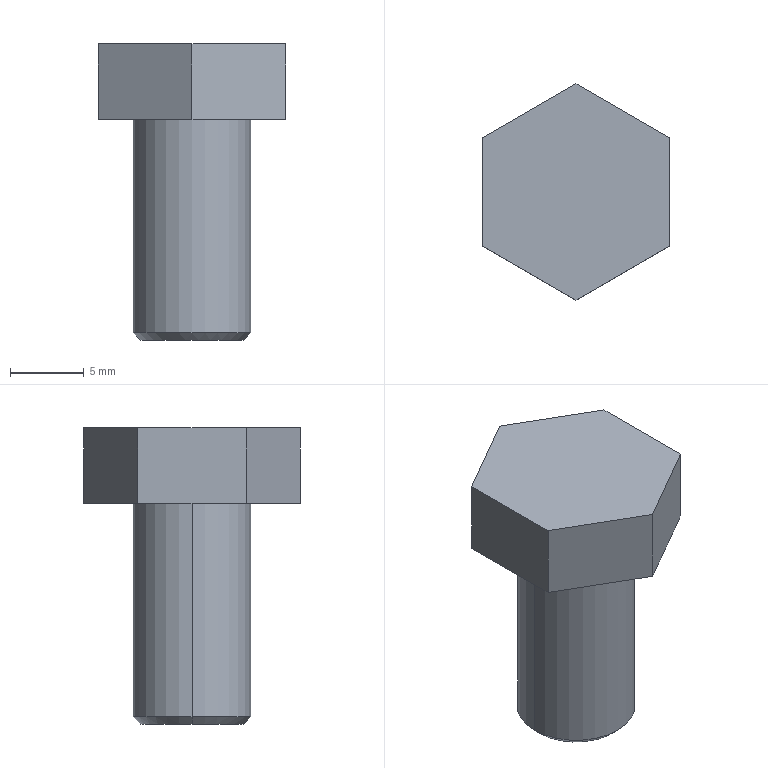Part | STEP file | Bulong M8_1.5F | 1 solid | 13 faces | box 12.73 x 14.699 x 20.15 mm | volume 1474 mm3 | plane 9 | cone 2 | cylinder 2 | commonest cylinder face diameters 8 x2
STEP:
#1=CARTESIAN_POINT('',(0.,0.,0.));
#2=DIRECTION('',(0.,0.,1.));
#3=DIRECTION('',(1.,0.,0.));
#4=AXIS2_PLACEMENT_3D('',#1,#2,#3);
#5=CARTESIAN_POINT('',(-3.5,0.,-15.));
#6=VERTEX_POINT('',#5);
#7=CARTESIAN_POINT('',(3.5,0.,-15.));
#8=VERTEX_POINT('',#7);
#9=CARTESIAN_POINT('',(0.,0.,-15.));
#10=DIRECTION('',(0.,0.,-1.));
#11=DIRECTION('',(-1.,0.,0.));
#12=AXIS2_PLACEMENT_3D('',#9,#10,#11);
#13=CIRCLE('',#12,3.5);
#14=CARTESIAN_POINT('',(0.,0.,-15.));
#15=DIRECTION('',(0.,0.,1.));
#16=DIRECTION('',(1.,0.,0.));
#17=AXIS2_PLACEMENT_3D('',#14,#15,#16);
#18=CONICAL_SURFACE('',#17,3.5,0.7854);
#19=CARTESIAN_POINT('',(3.142,0.));
#20=DIRECTION('',(-1.,0.));
#21=VECTOR('',#20,1.);
#22=LINE('',#19,#21);
#23=(GEOMETRIC_REPRESENTATION_CONTEXT(2)PARAMETRIC_REPRESENTATION_CONTEXT()REPRESENTATION_CONTEXT('',''));
#24=DEFINITIONAL_REPRESENTATION('',(#22),#23);
#25=PCURVE('',#18,#24);
#26=CARTESIAN_POINT('',(0.,0.,-15.));
#27=DIRECTION('',(0.,0.,-1.));
#28=DIRECTION('',(-1.,0.,0.));
#29=AXIS2_PLACEMENT_3D('',#26,#27,#28);
#30=PLANE('',#29);
#31=CARTESIAN_POINT('',(0.,0.));
#32=DIRECTION('',(1.,0.));
#33=AXIS2_PLACEMENT_2D('',#31,#32);
#34=CIRCLE('',#33,3.5);
#35=(GEOMETRIC_REPRESENTATION_CONTEXT(2)PARAMETRIC_REPRESENTATION_CONTEXT()REPRESENTATION_CONTEXT('',''));
#36=DEFINITIONAL_REPRESENTATION('',(#34),#35);
#37=PCURVE('',#30,#36);
#38=SURFACE_CURVE('',#13,(#25,#37),.PCURVE_S1.);
#39=EDGE_CURVE('',#6,#8,#38,.T.);
#40=ORIENTED_EDGE('',*,*,#39,.F.);
#41=CARTESIAN_POINT('',(-4.,0.,-14.5));
#42=VERTEX_POINT('',#41);
#43=CARTESIAN_POINT('',(-3.5,0.,-15.));
#44=DIRECTION('',(-0.7071,0.,0.7071));
#45=VECTOR('',#44,1.);
#46=LINE('',#43,#45);
#47=CARTESIAN_POINT('',(3.142,0.));
#48=DIRECTION('',(0.,1.));
#49=VECTOR('',#48,1.);
#50=LINE('',#47,#49);
#51=(GEOMETRIC_REPRESENTATION_CONTEXT(2)PARAMETRIC_REPRESENTATION_CONTEXT()REPRESENTATION_CONTEXT('',''));
#52=DEFINITIONAL_REPRESENTATION('',(#50),#51);
#53=PCURVE('',#18,#52);
#54=CARTESIAN_POINT('',(0.,0.,-15.));
#55=DIRECTION('',(0.,0.,1.));
#56=DIRECTION('',(1.,0.,0.));
#57=AXIS2_PLACEMENT_3D('',#54,#55,#56);
#58=CONICAL_SURFACE('',#57,3.5,0.7854);
#59=CARTESIAN_POINT('',(3.142,0.));
#60=DIRECTION('',(0.,1.));
#61=VECTOR('',#60,1.);
#62=LINE('',#59,#61);
#63=(GEOMETRIC_REPRESENTATION_CONTEXT(2)PARAMETRIC_REPRESENTATION_CONTEXT()REPRESENTATION_CONTEXT('',''));
#64=DEFINITIONAL_REPRESENTATION('',(#62),#63);
#65=PCURVE('',#58,#64);
#66=SURFACE_CURVE('',#46,(#53,#65),.PCURVE_S1.);
#67=EDGE_CURVE('',#6,#42,#66,.T.);
#68=ORIENTED_EDGE('',*,*,#67,.T.);
#69=CARTESIAN_POINT('',(4.,0.,-14.5));
#70=VERTEX_POINT('',#69);
#71=CARTESIAN_POINT('',(0.,0.,-14.5));
#72=DIRECTION('',(0.,0.,1.));
#73=DIRECTION('',(-1.,0.,0.));
#74=AXIS2_PLACEMENT_3D('',#71,#72,#73);
#75=CIRCLE('',#74,4.);
#76=CARTESIAN_POINT('',(-3.142,0.5));
#77=DIRECTION('',(1.,0.));
#78=VECTOR('',#77,1.);
#79=LINE('',#76,#78);
#80=(GEOMETRIC_REPRESENTATION_CONTEXT(2)PARAMETRIC_REPRESENTATION_CONTEXT()REPRESENTATION_CONTEXT('',''));
#81=DEFINITIONAL_REPRESENTATION('',(#79),#80);
#82=PCURVE('',#18,#81);
#83=CARTESIAN_POINT('',(0.,0.,-15.));
#84=DIRECTION('',(0.,0.,1.));
#85=DIRECTION('',(1.,0.,0.));
#86=AXIS2_PLACEMENT_3D('',#83,#84,#85);
#87=CYLINDRICAL_SURFACE('',#86,4.);
#88=CARTESIAN_POINT('',(-3.142,0.5));
#89=DIRECTION('',(1.,0.));
#90=VECTOR('',#89,1.);
#91=LINE('',#88,#90);
#92=(GEOMETRIC_REPRESENTATION_CONTEXT(2)PARAMETRIC_REPRESENTATION_CONTEXT()REPRESENTATION_CONTEXT('',''));
#93=DEFINITIONAL_REPRESENTATION('',(#91),#92);
#94=PCURVE('',#87,#93);
#95=SURFACE_CURVE('',#75,(#82,#94),.PCURVE_S1.);
#96=EDGE_CURVE('',#70,#42,#95,.T.);
#97=ORIENTED_EDGE('',*,*,#96,.F.);
#98=CARTESIAN_POINT('',(3.5,0.,-15.));
#99=DIRECTION('',(0.7071,0.,0.7071));
#100=VECTOR('',#99,1.);
#101=LINE('',#98,#100);
#102=CARTESIAN_POINT('',(0.,0.));
#103=DIRECTION('',(0.,1.));
#104=VECTOR('',#103,1.);
#105=LINE('',#102,#104);
#106=(GEOMETRIC_REPRESENTATION_CONTEXT(2)PARAMETRIC_REPRESENTATION_CONTEXT()REPRESENTATION_CONTEXT('',''));
#107=DEFINITIONAL_REPRESENTATION('',(#105),#106);
#108=PCURVE('',#18,#107);
#109=CARTESIAN_POINT('',(6.283,0.));
#110=DIRECTION('',(0.,1.));
#111=VECTOR('',#110,1.);
#112=LINE('',#109,#111);
#113=(GEOMETRIC_REPRESENTATION_CONTEXT(2)PARAMETRIC_REPRESENTATION_CONTEXT()REPRESENTATION_CONTEXT('',''));
#114=DEFINITIONAL_REPRESENTATION('',(#112),#113);
#115=PCURVE('',#58,#114);
#116=SURFACE_CURVE('',#101,(#108,#115),.PCURVE_S1.);
#117=EDGE_CURVE('',#8,#70,#116,.T.);
#118=ORIENTED_EDGE('',*,*,#117,.F.);
#119=EDGE_LOOP('',(#40,#68,#97,#118));
#120=FACE_BOUND('',#119,.T.);
#121=ADVANCED_FACE('',(#120),#18,.T.);
#122=ORIENTED_EDGE('',*,*,#96,.T.);
#123=CARTESIAN_POINT('',(-4.,0.,0.));
#124=VERTEX_POINT('',#123);
#125=CARTESIAN_POINT('',(-4.,0.,-15.));
#126=DIRECTION('',(0.,0.,1.));
#127=VECTOR('',#126,1.);
#128=LINE('',#125,#127);
#129=CARTESIAN_POINT('',(3.142,0.));
#130=DIRECTION('',(0.,1.));
#131=VECTOR('',#130,1.);
#132=LINE('',#129,#131);
#133=(GEOMETRIC_REPRESENTATION_CONTEXT(2)PARAMETRIC_REPRESENTATION_CONTEXT()REPRESENTATION_CONTEXT('',''));
#134=DEFINITIONAL_REPRESENTATION('',(#132),#133);
#135=PCURVE('',#87,#134);
#136=CARTESIAN_POINT('',(0.,0.,-15.));
#137=DIRECTION('',(0.,0.,1.));
#138=DIRECTION('',(1.,0.,0.));
#139=AXIS2_PLACEMENT_3D('',#136,#137,#138);
#140=CYLINDRICAL_SURFACE('',#139,4.);
#141=CARTESIAN_POINT('',(3.142,0.));
#142=DIRECTION('',(0.,1.));
#143=VECTOR('',#142,1.);
#144=LINE('',#141,#143);
#145=(GEOMETRIC_REPRESENTATION_CONTEXT(2)PARAMETRIC_REPRESENTATION_CONTEXT()REPRESENTATION_CONTEXT('',''));
#146=DEFINITIONAL_REPRESENTATION('',(#144),#145);
#147=PCURVE('',#140,#146);
#148=SURFACE_CURVE('',#128,(#135,#147),.PCURVE_S1.);
#149=EDGE_CURVE('',#42,#124,#148,.T.);
#150=ORIENTED_EDGE('',*,*,#149,.T.);
#151=CARTESIAN_POINT('',(4.,0.,0.));
#152=VERTEX_POINT('',#151);
#153=CARTESIAN_POINT('',(0.,0.,0.));
#154=DIRECTION('',(0.,0.,-1.));
#155=DIRECTION('',(1.,0.,0.));
#156=AXIS2_PLACEMENT_3D('',#153,#154,#155);
#157=CIRCLE('',#156,4.);
#158=CARTESIAN_POINT('',(6.283,15.));
#159=DIRECTION('',(-1.,0.));
#160=VECTOR('',#159,1.);
#161=LINE('',#158,#160);
#162=(GEOMETRIC_REPRESENTATION_CONTEXT(2)PARAMETRIC_REPRESENTATION_CONTEXT()REPRESENTATION_CONTEXT('',''));
#163=DEFINITIONAL_REPRESENTATION('',(#161),#162);
#164=PCURVE('',#87,#163);
#165=CARTESIAN_POINT('',(0.,0.,0.));
#166=DIRECTION('',(0.,0.,1.));
#167=DIRECTION('',(1.,0.,0.));
#168=AXIS2_PLACEMENT_3D('',#165,#166,#167);
#169=PLANE('',#168);
#170=CARTESIAN_POINT('',(4.,0.));
#171=CARTESIAN_POINT('',(4.,-6.928));
#172=CARTESIAN_POINT('',(-2.,-3.464));
#173=CARTESIAN_POINT('',(-8.,0.));
#174=CARTESIAN_POINT('',(-2.,3.464));
#175=CARTESIAN_POINT('',(4.,6.928));
#176=CARTESIAN_POINT('',(4.,0.));
#177=(BOUNDED_CURVE()B_SPLINE_CURVE(2,(#170,#171,#172,#173,#174,#175,#176),.UNSPECIFIED.,.T.,.F.)B_SPLINE_CURVE_WITH_KNOTS((1,2,2,2,2,1),(-2.094,0.,2.094,4.189,6.283,8.378),.UNSPECIFIED.)CURVE()GEOMETRIC_REPRESENTATION_ITEM()RATIONAL_B_SPLINE_CURVE((1.,0.5,1.,0.5,1.,0.5,1.))REPRESENTATION_ITEM(''));
#178=(GEOMETRIC_REPRESENTATION_CONTEXT(2)PARAMETRIC_REPRESENTATION_CONTEXT()REPRESENTATION_CONTEXT('',''));
#179=DEFINITIONAL_REPRESENTATION('',(#177),#178);
#180=PCURVE('',#169,#179);
#181=SURFACE_CURVE('',#157,(#164,#180),.PCURVE_S1.);
#182=EDGE_CURVE('',#124,#152,#181,.T.);
#183=ORIENTED_EDGE('',*,*,#182,.T.);
#184=CARTESIAN_POINT('',(4.,0.,-15.));
#185=DIRECTION('',(0.,0.,1.));
#186=VECTOR('',#185,1.);
#187=LINE('',#184,#186);
#188=CARTESIAN_POINT('',(0.,0.));
#189=DIRECTION('',(0.,1.));
#190=VECTOR('',#189,1.);
#191=LINE('',#188,#190);
#192=(GEOMETRIC_REPRESENTATION_CONTEXT(2)PARAMETRIC_REPRESENTATION_CONTEXT()REPRESENTATION_CONTEXT('',''));
#193=DEFINITIONAL_REPRESENTATION('',(#191),#192);
#194=PCURVE('',#87,#193);
#195=CARTESIAN_POINT('',(6.283,0.));
#196=DIRECTION('',(0.,1.));
#197=VECTOR('',#196,1.);
#198=LINE('',#195,#197);
#199=(GEOMETRIC_REPRESENTATION_CONTEXT(2)PARAMETRIC_REPRESENTATION_CONTEXT()REPRESENTATION_CONTEXT('',''));
#200=DEFINITIONAL_REPRESENTATION('',(#198),#199);
#201=PCURVE('',#140,#200);
#202=SURFACE_CURVE('',#187,(#194,#201),.PCURVE_S1.);
#203=EDGE_CURVE('',#70,#152,#202,.T.);
#204=ORIENTED_EDGE('',*,*,#203,.F.);
#205=EDGE_LOOP('',(#122,#150,#183,#204));
#206=FACE_BOUND('',#205,.T.);
#207=ADVANCED_FACE('',(#206),#87,.T.);
#208=CARTESIAN_POINT('',(6.365,3.675,0.));
#209=VERTEX_POINT('',#208);
#210=CARTESIAN_POINT('',(0.,7.35,0.));
#211=VERTEX_POINT('',#210);
#212=CARTESIAN_POINT('',(6.365,3.675,0.));
#213=DIRECTION('',(-0.866,0.5,0.));
#214=VECTOR('',#213,1.);
#215=LINE('',#212,#214);
#216=CARTESIAN_POINT('',(6.365,3.675));
#217=DIRECTION('',(-0.866,0.5));
#218=VECTOR('',#217,1.);
#219=LINE('',#216,#218);
#220=(GEOMETRIC_REPRESENTATION_CONTEXT(2)PARAMETRIC_REPRESENTATION_CONTEXT()REPRESENTATION_CONTEXT('',''));
#221=DEFINITIONAL_REPRESENTATION('',(#219),#220);
#222=PCURVE('',#169,#221);
#223=CARTESIAN_POINT('',(6.365,3.675,5.15));
#224=DIRECTION('',(-0.5,-0.866,0.));
#225=DIRECTION('',(0.866,-0.5,0.));
#226=AXIS2_PLACEMENT_3D('',#223,#224,#225);
#227=PLANE('',#226);
#228=CARTESIAN_POINT('',(0.,-5.15));
#229=DIRECTION('',(-1.,0.));
#230=VECTOR('',#229,1.);
#231=LINE('',#228,#230);
#232=(GEOMETRIC_REPRESENTATION_CONTEXT(2)PARAMETRIC_REPRESENTATION_CONTEXT()REPRESENTATION_CONTEXT('',''));
#233=DEFINITIONAL_REPRESENTATION('',(#231),#232);
#234=PCURVE('',#227,#233);
#235=SURFACE_CURVE('',#215,(#222,#234),.PCURVE_S1.);
#236=EDGE_CURVE('',#209,#211,#235,.T.);
#237=ORIENTED_EDGE('',*,*,#236,.F.);
#238=CARTESIAN_POINT('',(6.365,-3.675,0.));
#239=VERTEX_POINT('',#238);
#240=CARTESIAN_POINT('',(6.365,-3.675,0.));
#241=DIRECTION('',(0.,1.,0.));
#242=VECTOR('',#241,1.);
#243=LINE('',#240,#242);
#244=CARTESIAN_POINT('',(6.365,-3.675));
#245=DIRECTION('',(0.,1.));
#246=VECTOR('',#245,1.);
#247=LINE('',#244,#246);
#248=(GEOMETRIC_REPRESENTATION_CONTEXT(2)PARAMETRIC_REPRESENTATION_CONTEXT()REPRESENTATION_CONTEXT('',''));
#249=DEFINITIONAL_REPRESENTATION('',(#247),#248);
#250=PCURVE('',#169,#249);
#251=CARTESIAN_POINT('',(6.365,-3.675,5.15));
#252=DIRECTION('',(-1.,0.,0.));
#253=DIRECTION('',(0.,-1.,0.));
#254=AXIS2_PLACEMENT_3D('',#251,#252,#253);
#255=PLANE('',#254);
#256=CARTESIAN_POINT('',(0.,-5.15));
#257=DIRECTION('',(-1.,0.));
#258=VECTOR('',#257,1.);
#259=LINE('',#256,#258);
#260=(GEOMETRIC_REPRESENTATION_CONTEXT(2)PARAMETRIC_REPRESENTATION_CONTEXT()REPRESENTATION_CONTEXT('',''));
#261=DEFINITIONAL_REPRESENTATION('',(#259),#260);
#262=PCURVE('',#255,#261);
#263=SURFACE_CURVE('',#243,(#250,#262),.PCURVE_S1.);
#264=EDGE_CURVE('',#239,#209,#263,.T.);
#265=ORIENTED_EDGE('',*,*,#264,.F.);
#266=CARTESIAN_POINT('',(0.,-7.35,0.));
#267=VERTEX_POINT('',#266);
#268=CARTESIAN_POINT('',(0.,-7.35,0.));
#269=DIRECTION('',(0.866,0.5,0.));
#270=VECTOR('',#269,1.);
#271=LINE('',#268,#270);
#272=CARTESIAN_POINT('',(0.,-7.35));
#273=DIRECTION('',(0.866,0.5));
#274=VECTOR('',#273,1.);
#275=LINE('',#272,#274);
#276=(GEOMETRIC_REPRESENTATION_CONTEXT(2)PARAMETRIC_REPRESENTATION_CONTEXT()REPRESENTATION_CONTEXT('',''));
#277=DEFINITIONAL_REPRESENTATION('',(#275),#276);
#278=PCURVE('',#169,#277);
#279=CARTESIAN_POINT('',(0.,-7.35,5.15));
#280=DIRECTION('',(-0.5,0.866,0.));
#281=DIRECTION('',(-0.866,-0.5,0.));
#282=AXIS2_PLACEMENT_3D('',#279,#280,#281);
#283=PLANE('',#282);
#284=CARTESIAN_POINT('',(0.,-5.15));
#285=DIRECTION('',(-1.,0.));
#286=VECTOR('',#285,1.);
#287=LINE('',#284,#286);
#288=(GEOMETRIC_REPRESENTATION_CONTEXT(2)PARAMETRIC_REPRESENTATION_CONTEXT()REPRESENTATION_CONTEXT('',''));
#289=DEFINITIONAL_REPRESENTATION('',(#287),#288);
#290=PCURVE('',#283,#289);
#291=SURFACE_CURVE('',#271,(#278,#290),.PCURVE_S1.);
#292=EDGE_CURVE('',#267,#239,#291,.T.);
#293=ORIENTED_EDGE('',*,*,#292,.F.);
#294=CARTESIAN_POINT('',(-6.365,-3.675,0.));
#295=VERTEX_POINT('',#294);
#296=CARTESIAN_POINT('',(-6.365,-3.675,0.));
#297=DIRECTION('',(0.866,-0.5,0.));
#298=VECTOR('',#297,1.);
#299=LINE('',#296,#298);
#300=CARTESIAN_POINT('',(-6.365,-3.675));
#301=DIRECTION('',(0.866,-0.5));
#302=VECTOR('',#301,1.);
#303=LINE('',#300,#302);
#304=(GEOMETRIC_REPRESENTATION_CONTEXT(2)PARAMETRIC_REPRESENTATION_CONTEXT()REPRESENTATION_CONTEXT('',''));
#305=DEFINITIONAL_REPRESENTATION('',(#303),#304);
#306=PCURVE('',#169,#305);
#307=CARTESIAN_POINT('',(-6.365,-3.675,5.15));
#308=DIRECTION('',(0.5,0.866,0.));
#309=DIRECTION('',(-0.866,0.5,0.));
#310=AXIS2_PLACEMENT_3D('',#307,#308,#309);
#311=PLANE('',#310);
#312=CARTESIAN_POINT('',(0.,-5.15));
#313=DIRECTION('',(-1.,0.));
#314=VECTOR('',#313,1.);
#315=LINE('',#312,#314);
#316=(GEOMETRIC_REPRESENTATION_CONTEXT(2)PARAMETRIC_REPRESENTATION_CONTEXT()REPRESENTATION_CONTEXT('',''));
#317=DEFINITIONAL_REPRESENTATION('',(#315),#316);
#318=PCURVE('',#311,#317);
#319=SURFACE_CURVE('',#299,(#306,#318),.PCURVE_S1.);
#320=EDGE_CURVE('',#295,#267,#319,.T.);
#321=ORIENTED_EDGE('',*,*,#320,.F.);
#322=CARTESIAN_POINT('',(-6.365,3.675,0.));
#323=VERTEX_POINT('',#322);
#324=CARTESIAN_POINT('',(-6.365,3.675,0.));
#325=DIRECTION('',(0.,-1.,0.));
#326=VECTOR('',#325,1.);
#327=LINE('',#324,#326);
#328=CARTESIAN_POINT('',(-6.365,3.675));
#329=DIRECTION('',(0.,-1.));
#330=VECTOR('',#329,1.);
#331=LINE('',#328,#330);
#332=(GEOMETRIC_REPRESENTATION_CONTEXT(2)PARAMETRIC_REPRESENTATION_CONTEXT()REPRESENTATION_CONTEXT('',''));
#333=DEFINITIONAL_REPRESENTATION('',(#331),#332);
#334=PCURVE('',#169,#333);
#335=CARTESIAN_POINT('',(-6.365,3.675,5.15));
#336=DIRECTION('',(1.,0.,0.));
#337=DIRECTION('',(0.,0.,-1.));
#338=AXIS2_PLACEMENT_3D('',#335,#336,#337);
#339=PLANE('',#338);
#340=CARTESIAN_POINT('',(5.15,0.));
#341=DIRECTION('',(0.,-1.));
#342=VECTOR('',#341,1.);
#343=LINE('',#340,#342);
#344=(GEOMETRIC_REPRESENTATION_CONTEXT(2)PARAMETRIC_REPRESENTATION_CONTEXT()REPRESENTATION_CONTEXT('',''));
#345=DEFINITIONAL_REPRESENTATION('',(#343),#344);
#346=PCURVE('',#339,#345);
#347=SURFACE_CURVE('',#327,(#334,#346),.PCURVE_S1.);
#348=EDGE_CURVE('',#323,#295,#347,.T.);
#349=ORIENTED_EDGE('',*,*,#348,.F.);
#350=CARTESIAN_POINT('',(0.,7.35,0.));
#351=DIRECTION('',(-0.866,-0.5,0.));
#352=VECTOR('',#351,1.);
#353=LINE('',#350,#352);
#354=CARTESIAN_POINT('',(0.,7.35));
#355=DIRECTION('',(-0.866,-0.5));
#356=VECTOR('',#355,1.);
#357=LINE('',#354,#356);
#358=(GEOMETRIC_REPRESENTATION_CONTEXT(2)PARAMETRIC_REPRESENTATION_CONTEXT()REPRESENTATION_CONTEXT('',''));
#359=DEFINITIONAL_REPRESENTATION('',(#357),#358);
#360=PCURVE('',#169,#359);
#361=CARTESIAN_POINT('',(0.,7.35,5.15));
#362=DIRECTION('',(0.5,-0.866,0.));
#363=DIRECTION('',(0.866,0.5,0.));
#364=AXIS2_PLACEMENT_3D('',#361,#362,#363);
#365=PLANE('',#364);
#366=CARTESIAN_POINT('',(0.,-5.15));
#367=DIRECTION('',(-1.,0.));
#368=VECTOR('',#367,1.);
#369=LINE('',#366,#368);
#370=(GEOMETRIC_REPRESENTATION_CONTEXT(2)PARAMETRIC_REPRESENTATION_CONTEXT()REPRESENTATION_CONTEXT('',''));
#371=DEFINITIONAL_REPRESENTATION('',(#369),#370);
#372=PCURVE('',#365,#371);
#373=SURFACE_CURVE('',#353,(#360,#372),.PCURVE_S1.);
#374=EDGE_CURVE('',#211,#323,#373,.T.);
#375=ORIENTED_EDGE('',*,*,#374,.F.);
#376=EDGE_LOOP('',(#237,#265,#293,#321,#349,#375));
#377=FACE_BOUND('',#376,.T.);
#378=CARTESIAN_POINT('',(0.,0.,0.));
#379=DIRECTION('',(0.,0.,-1.));
#380=DIRECTION('',(1.,0.,0.));
#381=AXIS2_PLACEMENT_3D('',#378,#379,#380);
#382=CIRCLE('',#381,4.);
#383=CARTESIAN_POINT('',(4.,0.));
#384=CARTESIAN_POINT('',(4.,-6.928));
#385=CARTESIAN_POINT('',(-2.,-3.464));
#386=CARTESIAN_POINT('',(-8.,0.));
#387=CARTESIAN_POINT('',(-2.,3.464));
#388=CARTESIAN_POINT('',(4.,6.928));
#389=CARTESIAN_POINT('',(4.,0.));
#390=(BOUNDED_CURVE()B_SPLINE_CURVE(2,(#383,#384,#385,#386,#387,#388,#389),.UNSPECIFIED.,.T.,.F.)B_SPLINE_CURVE_WITH_KNOTS((1,2,2,2,2,1),(-2.094,0.,2.094,4.189,6.283,8.378),.UNSPECIFIED.)CURVE()GEOMETRIC_REPRESENTATION_ITEM()RATIONAL_B_SPLINE_CURVE((1.,0.5,1.,0.5,1.,0.5,1.))REPRESENTATION_ITEM(''));
#391=(GEOMETRIC_REPRESENTATION_CONTEXT(2)PARAMETRIC_REPRESENTATION_CONTEXT()REPRESENTATION_CONTEXT('',''));
#392=DEFINITIONAL_REPRESENTATION('',(#390),#391);
#393=PCURVE('',#169,#392);
#394=CARTESIAN_POINT('',(6.283,15.));
#395=DIRECTION('',(-1.,0.));
#396=VECTOR('',#395,1.);
#397=LINE('',#394,#396);
#398=(GEOMETRIC_REPRESENTATION_CONTEXT(2)PARAMETRIC_REPRESENTATION_CONTEXT()REPRESENTATION_CONTEXT('',''));
#399=DEFINITIONAL_REPRESENTATION('',(#397),#398);
#400=PCURVE('',#140,#399);
#401=SURFACE_CURVE('',#382,(#393,#400),.PCURVE_S1.);
#402=EDGE_CURVE('',#152,#124,#401,.T.);
#403=ORIENTED_EDGE('',*,*,#402,.F.);
#404=ORIENTED_EDGE('',*,*,#182,.F.);
#405=EDGE_LOOP('',(#403,#404));
#406=FACE_BOUND('',#405,.T.);
#407=ADVANCED_FACE('',(#377,#406),#169,.F.);
#408=ORIENTED_EDGE('',*,*,#236,.T.);
#409=CARTESIAN_POINT('',(0.,7.35,5.15));
#410=VERTEX_POINT('',#409);
#411=CARTESIAN_POINT('',(0.,7.35,5.15));
#412=DIRECTION('',(0.,0.,-1.));
#413=VECTOR('',#412,1.);
#414=LINE('',#411,#413);
#415=CARTESIAN_POINT('',(-7.35,0.));
#416=DIRECTION('',(0.,-1.));
#417=VECTOR('',#416,1.);
#418=LINE('',#415,#417);
#419=(GEOMETRIC_REPRESENTATION_CONTEXT(2)PARAMETRIC_REPRESENTATION_CONTEXT()REPRESENTATION_CONTEXT('',''));
#420=DEFINITIONAL_REPRESENTATION('',(#418),#419);
#421=PCURVE('',#227,#420);
#422=CARTESIAN_POINT('',(0.,0.));
#423=DIRECTION('',(0.,-1.));
#424=VECTOR('',#423,1.);
#425=LINE('',#422,#424);
#426=(GEOMETRIC_REPRESENTATION_CONTEXT(2)PARAMETRIC_REPRESENTATION_CONTEXT()REPRESENTATION_CONTEXT('',''));
#427=DEFINITIONAL_REPRESENTATION('',(#425),#426);
#428=PCURVE('',#365,#427);
#429=SURFACE_CURVE('',#414,(#421,#428),.PCURVE_S1.);
#430=EDGE_CURVE('',#410,#211,#429,.T.);
#431=ORIENTED_EDGE('',*,*,#430,.F.);
#432=CARTESIAN_POINT('',(6.365,3.675,5.15));
#433=VERTEX_POINT('',#432);
#434=CARTESIAN_POINT('',(6.365,3.675,5.15));
#435=DIRECTION('',(-0.866,0.5,0.));
#436=VECTOR('',#435,1.);
#437=LINE('',#434,#436);
#438=CARTESIAN_POINT('',(0.,0.));
#439=DIRECTION('',(-1.,0.));
#440=VECTOR('',#439,1.);
#441=LINE('',#438,#440);
#442=(GEOMETRIC_REPRESENTATION_CONTEXT(2)PARAMETRIC_REPRESENTATION_CONTEXT()REPRESENTATION_CONTEXT('',''));
#443=DEFINITIONAL_REPRESENTATION('',(#441),#442);
#444=PCURVE('',#227,#443);
#445=CARTESIAN_POINT('',(0.,0.,5.15));
#446=DIRECTION('',(0.,0.,1.));
#447=DIRECTION('',(1.,0.,0.));
#448=AXIS2_PLACEMENT_3D('',#445,#446,#447);
#449=PLANE('',#448);
#450=CARTESIAN_POINT('',(6.365,3.675));
#451=DIRECTION('',(-0.866,0.5));
#452=VECTOR('',#451,1.);
#453=LINE('',#450,#452);
#454=(GEOMETRIC_REPRESENTATION_CONTEXT(2)PARAMETRIC_REPRESENTATION_CONTEXT()REPRESENTATION_CONTEXT('',''));
#455=DEFINITIONAL_REPRESENTATION('',(#453),#454);
#456=PCURVE('',#449,#455);
#457=SURFACE_CURVE('',#437,(#444,#456),.PCURVE_S1.);
#458=EDGE_CURVE('',#433,#410,#457,.T.);
#459=ORIENTED_EDGE('',*,*,#458,.F.);
#460=CARTESIAN_POINT('',(6.365,3.675,5.15));
#461=DIRECTION('',(0.,0.,-1.));
#462=VECTOR('',#461,1.);
#463=LINE('',#460,#462);
#464=CARTESIAN_POINT('',(0.,0.));
#465=DIRECTION('',(0.,-1.));
#466=VECTOR('',#465,1.);
#467=LINE('',#464,#466);
#468=(GEOMETRIC_REPRESENTATION_CONTEXT(2)PARAMETRIC_REPRESENTATION_CONTEXT()REPRESENTATION_CONTEXT('',''));
#469=DEFINITIONAL_REPRESENTATION('',(#467),#468);
#470=PCURVE('',#227,#469);
#471=CARTESIAN_POINT('',(-7.35,0.));
#472=DIRECTION('',(0.,-1.));
#473=VECTOR('',#472,1.);
#474=LINE('',#471,#473);
#475=(GEOMETRIC_REPRESENTATION_CONTEXT(2)PARAMETRIC_REPRESENTATION_CONTEXT()REPRESENTATION_CONTEXT('',''));
#476=DEFINITIONAL_REPRESENTATION('',(#474),#475);
#477=PCURVE('',#255,#476);
#478=SURFACE_CURVE('',#463,(#470,#477),.PCURVE_S1.);
#479=EDGE_CURVE('',#433,#209,#478,.T.);
#480=ORIENTED_EDGE('',*,*,#479,.T.);
#481=EDGE_LOOP('',(#408,#431,#459,#480));
#482=FACE_BOUND('',#481,.T.);
#483=ADVANCED_FACE('',(#482),#227,.F.);
#484=ORIENTED_EDGE('',*,*,#374,.T.);
#485=CARTESIAN_POINT('',(-6.365,3.675,5.15));
#486=VERTEX_POINT('',#485);
#487=CARTESIAN_POINT('',(-6.365,3.675,5.15));
#488=DIRECTION('',(0.,0.,-1.));
#489=VECTOR('',#488,1.);
#490=LINE('',#487,#489);
#491=CARTESIAN_POINT('',(-7.35,0.));
#492=DIRECTION('',(0.,-1.));
#493=VECTOR('',#492,1.);
#494=LINE('',#491,#493);
#495=(GEOMETRIC_REPRESENTATION_CONTEXT(2)PARAMETRIC_REPRESENTATION_CONTEXT()REPRESENTATION_CONTEXT('',''));
#496=DEFINITIONAL_REPRESENTATION('',(#494),#495);
#497=PCURVE('',#365,#496);
#498=CARTESIAN_POINT('',(0.,0.));
#499=DIRECTION('',(1.,0.));
#500=VECTOR('',#499,1.);
#501=LINE('',#498,#500);
#502=(GEOMETRIC_REPRESENTATION_CONTEXT(2)PARAMETRIC_REPRESENTATION_CONTEXT()REPRESENTATION_CONTEXT('',''));
#503=DEFINITIONAL_REPRESENTATION('',(#501),#502);
#504=PCURVE('',#339,#503);
#505=SURFACE_CURVE('',#490,(#497,#504),.PCURVE_S1.);
#506=EDGE_CURVE('',#486,#323,#505,.T.);
#507=ORIENTED_EDGE('',*,*,#506,.F.);
#508=CARTESIAN_POINT('',(0.,7.35,5.15));
#509=DIRECTION('',(-0.866,-0.5,0.));
#510=VECTOR('',#509,1.);
#511=LINE('',#508,#510);
#512=CARTESIAN_POINT('',(0.,0.));
#513=DIRECTION('',(-1.,0.));
#514=VECTOR('',#513,1.);
#515=LINE('',#512,#514);
#516=(GEOMETRIC_REPRESENTATION_CONTEXT(2)PARAMETRIC_REPRESENTATION_CONTEXT()REPRESENTATION_CONTEXT('',''));
#517=DEFINITIONAL_REPRESENTATION('',(#515),#516);
#518=PCURVE('',#365,#517);
#519=CARTESIAN_POINT('',(0.,7.35));
#520=DIRECTION('',(-0.866,-0.5));
#521=VECTOR('',#520,1.);
#522=LINE('',#519,#521);
#523=(GEOMETRIC_REPRESENTATION_CONTEXT(2)PARAMETRIC_REPRESENTATION_CONTEXT()REPRESENTATION_CONTEXT('',''));
#524=DEFINITIONAL_REPRESENTATION('',(#522),#523);
#525=PCURVE('',#449,#524);
#526=SURFACE_CURVE('',#511,(#518,#525),.PCURVE_S1.);
#527=EDGE_CURVE('',#410,#486,#526,.T.);
#528=ORIENTED_EDGE('',*,*,#527,.F.);
#529=ORIENTED_EDGE('',*,*,#430,.T.);
#530=EDGE_LOOP('',(#484,#507,#528,#529));
#531=FACE_BOUND('',#530,.T.);
#532=ADVANCED_FACE('',(#531),#365,.F.);
#533=ORIENTED_EDGE('',*,*,#348,.T.);
#534=CARTESIAN_POINT('',(-6.365,-3.675,5.15));
#535=VERTEX_POINT('',#534);
#536=CARTESIAN_POINT('',(-6.365,-3.675,5.15));
#537=DIRECTION('',(0.,0.,-1.));
#538=VECTOR('',#537,1.);
#539=LINE('',#536,#538);
#540=CARTESIAN_POINT('',(0.,-7.35));
#541=DIRECTION('',(1.,0.));
#542=VECTOR('',#541,1.);
#543=LINE('',#540,#542);
#544=(GEOMETRIC_REPRESENTATION_CONTEXT(2)PARAMETRIC_REPRESENTATION_CONTEXT()REPRESENTATION_CONTEXT('',''));
#545=DEFINITIONAL_REPRESENTATION('',(#543),#544);
#546=PCURVE('',#339,#545);
#547=CARTESIAN_POINT('',(0.,0.));
#548=DIRECTION('',(0.,-1.));
#549=VECTOR('',#548,1.);
#550=LINE('',#547,#549);
#551=(GEOMETRIC_REPRESENTATION_CONTEXT(2)PARAMETRIC_REPRESENTATION_CONTEXT()REPRESENTATION_CONTEXT('',''));
#552=DEFINITIONAL_REPRESENTATION('',(#550),#551);
#553=PCURVE('',#311,#552);
#554=SURFACE_CURVE('',#539,(#546,#553),.PCURVE_S1.);
#555=EDGE_CURVE('',#535,#295,#554,.T.);
#556=ORIENTED_EDGE('',*,*,#555,.F.);
#557=CARTESIAN_POINT('',(-6.365,3.675,5.15));
#558=DIRECTION('',(0.,-1.,0.));
#559=VECTOR('',#558,1.);
#560=LINE('',#557,#559);
#561=CARTESIAN_POINT('',(0.,0.));
#562=DIRECTION('',(0.,-1.));
#563=VECTOR('',#562,1.);
#564=LINE('',#561,#563);
#565=(GEOMETRIC_REPRESENTATION_CONTEXT(2)PARAMETRIC_REPRESENTATION_CONTEXT()REPRESENTATION_CONTEXT('',''));
#566=DEFINITIONAL_REPRESENTATION('',(#564),#565);
#567=PCURVE('',#339,#566);
#568=CARTESIAN_POINT('',(-6.365,3.675));
#569=DIRECTION('',(0.,-1.));
#570=VECTOR('',#569,1.);
#571=LINE('',#568,#570);
#572=(GEOMETRIC_REPRESENTATION_CONTEXT(2)PARAMETRIC_REPRESENTATION_CONTEXT()REPRESENTATION_CONTEXT('',''));
#573=DEFINITIONAL_REPRESENTATION('',(#571),#572);
#574=PCURVE('',#449,#573);
#575=SURFACE_CURVE('',#560,(#567,#574),.PCURVE_S1.);
#576=EDGE_CURVE('',#486,#535,#575,.T.);
#577=ORIENTED_EDGE('',*,*,#576,.F.);
#578=ORIENTED_EDGE('',*,*,#506,.T.);
#579=EDGE_LOOP('',(#533,#556,#577,#578));
#580=FACE_BOUND('',#579,.T.);
#581=ADVANCED_FACE('',(#580),#339,.F.);
#582=ORIENTED_EDGE('',*,*,#320,.T.);
#583=CARTESIAN_POINT('',(0.,-7.35,5.15));
#584=VERTEX_POINT('',#583);
#585=CARTESIAN_POINT('',(0.,-7.35,5.15));
#586=DIRECTION('',(0.,0.,-1.));
#587=VECTOR('',#586,1.);
#588=LINE('',#585,#587);
#589=CARTESIAN_POINT('',(-7.35,0.));
#590=DIRECTION('',(0.,-1.));
#591=VECTOR('',#590,1.);
#592=LINE('',#589,#591);
#593=(GEOMETRIC_REPRESENTATION_CONTEXT(2)PARAMETRIC_REPRESENTATION_CONTEXT()REPRESENTATION_CONTEXT('',''));
#594=DEFINITIONAL_REPRESENTATION('',(#592),#593);
#595=PCURVE('',#311,#594);
#596=CARTESIAN_POINT('',(0.,0.));
#597=DIRECTION('',(0.,-1.));
#598=VECTOR('',#597,1.);
#599=LINE('',#596,#598);
#600=(GEOMETRIC_REPRESENTATION_CONTEXT(2)PARAMETRIC_REPRESENTATION_CONTEXT()REPRESENTATION_CONTEXT('',''));
#601=DEFINITIONAL_REPRESENTATION('',(#599),#600);
#602=PCURVE('',#283,#601);
#603=SURFACE_CURVE('',#588,(#595,#602),.PCURVE_S1.);
#604=EDGE_CURVE('',#584,#267,#603,.T.);
#605=ORIENTED_EDGE('',*,*,#604,.F.);
#606=CARTESIAN_POINT('',(-6.365,-3.675,5.15));
#607=DIRECTION('',(0.866,-0.5,0.));
#608=VECTOR('',#607,1.);
#609=LINE('',#606,#608);
#610=CARTESIAN_POINT('',(0.,0.));
#611=DIRECTION('',(-1.,0.));
#612=VECTOR('',#611,1.);
#613=LINE('',#610,#612);
#614=(GEOMETRIC_REPRESENTATION_CONTEXT(2)PARAMETRIC_REPRESENTATION_CONTEXT()REPRESENTATION_CONTEXT('',''));
#615=DEFINITIONAL_REPRESENTATION('',(#613),#614);
#616=PCURVE('',#311,#615);
#617=CARTESIAN_POINT('',(-6.365,-3.675));
#618=DIRECTION('',(0.866,-0.5));
#619=VECTOR('',#618,1.);
#620=LINE('',#617,#619);
#621=(GEOMETRIC_REPRESENTATION_CONTEXT(2)PARAMETRIC_REPRESENTATION_CONTEXT()REPRESENTATION_CONTEXT('',''));
#622=DEFINITIONAL_REPRESENTATION('',(#620),#621);
#623=PCURVE('',#449,#622);
#624=SURFACE_CURVE('',#609,(#616,#623),.PCURVE_S1.);
#625=EDGE_CURVE('',#535,#584,#624,.T.);
#626=ORIENTED_EDGE('',*,*,#625,.F.);
#627=ORIENTED_EDGE('',*,*,#555,.T.);
#628=EDGE_LOOP('',(#582,#605,#626,#627));
#629=FACE_BOUND('',#628,.T.);
#630=ADVANCED_FACE('',(#629),#311,.F.);
#631=ORIENTED_EDGE('',*,*,#292,.T.);
#632=CARTESIAN_POINT('',(6.365,-3.675,5.15));
#633=VERTEX_POINT('',#632);
#634=CARTESIAN_POINT('',(6.365,-3.675,5.15));
#635=DIRECTION('',(0.,0.,-1.));
#636=VECTOR('',#635,1.);
#637=LINE('',#634,#636);
#638=CARTESIAN_POINT('',(-7.35,0.));
#639=DIRECTION('',(0.,-1.));
#640=VECTOR('',#639,1.);
#641=LINE('',#638,#640);
#642=(GEOMETRIC_REPRESENTATION_CONTEXT(2)PARAMETRIC_REPRESENTATION_CONTEXT()REPRESENTATION_CONTEXT('',''));
#643=DEFINITIONAL_REPRESENTATION('',(#641),#642);
#644=PCURVE('',#283,#643);
#645=CARTESIAN_POINT('',(0.,0.));
#646=DIRECTION('',(0.,-1.));
#647=VECTOR('',#646,1.);
#648=LINE('',#645,#647);
#649=(GEOMETRIC_REPRESENTATION_CONTEXT(2)PARAMETRIC_REPRESENTATION_CONTEXT()REPRESENTATION_CONTEXT('',''));
#650=DEFINITIONAL_REPRESENTATION('',(#648),#649);
#651=PCURVE('',#255,#650);
#652=SURFACE_CURVE('',#637,(#644,#651),.PCURVE_S1.);
#653=EDGE_CURVE('',#633,#239,#652,.T.);
#654=ORIENTED_EDGE('',*,*,#653,.F.);
#655=CARTESIAN_POINT('',(0.,-7.35,5.15));
#656=DIRECTION('',(0.866,0.5,0.));
#657=VECTOR('',#656,1.);
#658=LINE('',#655,#657);
#659=CARTESIAN_POINT('',(0.,0.));
#660=DIRECTION('',(-1.,0.));
#661=VECTOR('',#660,1.);
#662=LINE('',#659,#661);
#663=(GEOMETRIC_REPRESENTATION_CONTEXT(2)PARAMETRIC_REPRESENTATION_CONTEXT()REPRESENTATION_CONTEXT('',''));
#664=DEFINITIONAL_REPRESENTATION('',(#662),#663);
#665=PCURVE('',#283,#664);
#666=CARTESIAN_POINT('',(0.,-7.35));
#667=DIRECTION('',(0.866,0.5));
#668=VECTOR('',#667,1.);
#669=LINE('',#666,#668);
#670=(GEOMETRIC_REPRESENTATION_CONTEXT(2)PARAMETRIC_REPRESENTATION_CONTEXT()REPRESENTATION_CONTEXT('',''));
#671=DEFINITIONAL_REPRESENTATION('',(#669),#670);
#672=PCURVE('',#449,#671);
#673=SURFACE_CURVE('',#658,(#665,#672),.PCURVE_S1.);
#674=EDGE_CURVE('',#584,#633,#673,.T.);
#675=ORIENTED_EDGE('',*,*,#674,.F.);
#676=ORIENTED_EDGE('',*,*,#604,.T.);
#677=EDGE_LOOP('',(#631,#654,#675,#676));
#678=FACE_BOUND('',#677,.T.);
#679=ADVANCED_FACE('',(#678),#283,.F.);
#680=ORIENTED_EDGE('',*,*,#264,.T.);
#681=ORIENTED_EDGE('',*,*,#479,.F.);
#682=CARTESIAN_POINT('',(6.365,-3.675,5.15));
#683=DIRECTION('',(0.,1.,0.));
#684=VECTOR('',#683,1.);
#685=LINE('',#682,#684);
#686=CARTESIAN_POINT('',(0.,0.));
#687=DIRECTION('',(-1.,0.));
#688=VECTOR('',#687,1.);
#689=LINE('',#686,#688);
#690=(GEOMETRIC_REPRESENTATION_CONTEXT(2)PARAMETRIC_REPRESENTATION_CONTEXT()REPRESENTATION_CONTEXT('',''));
#691=DEFINITIONAL_REPRESENTATION('',(#689),#690);
#692=PCURVE('',#255,#691);
#693=CARTESIAN_POINT('',(6.365,-3.675));
#694=DIRECTION('',(0.,1.));
#695=VECTOR('',#694,1.);
#696=LINE('',#693,#695);
#697=(GEOMETRIC_REPRESENTATION_CONTEXT(2)PARAMETRIC_REPRESENTATION_CONTEXT()REPRESENTATION_CONTEXT('',''));
#698=DEFINITIONAL_REPRESENTATION('',(#696),#697);
#699=PCURVE('',#449,#698);
#700=SURFACE_CURVE('',#685,(#692,#699),.PCURVE_S1.);
#701=EDGE_CURVE('',#633,#433,#700,.T.);
#702=ORIENTED_EDGE('',*,*,#701,.F.);
#703=ORIENTED_EDGE('',*,*,#653,.T.);
#704=EDGE_LOOP('',(#680,#681,#702,#703));
#705=FACE_BOUND('',#704,.T.);
#706=ADVANCED_FACE('',(#705),#255,.F.);
#707=ORIENTED_EDGE('',*,*,#458,.T.);
#708=ORIENTED_EDGE('',*,*,#527,.T.);
#709=ORIENTED_EDGE('',*,*,#576,.T.);
#710=ORIENTED_EDGE('',*,*,#625,.T.);
#711=ORIENTED_EDGE('',*,*,#674,.T.);
#712=ORIENTED_EDGE('',*,*,#701,.T.);
#713=EDGE_LOOP('',(#707,#708,#709,#710,#711,#712));
#714=FACE_BOUND('',#713,.T.);
#715=ADVANCED_FACE('',(#714),#449,.T.);
#716=ORIENTED_EDGE('',*,*,#149,.F.);
#717=CARTESIAN_POINT('',(0.,0.,-14.5));
#718=DIRECTION('',(0.,0.,1.));
#719=DIRECTION('',(-1.,0.,0.));
#720=AXIS2_PLACEMENT_3D('',#717,#718,#719);
#721=CIRCLE('',#720,4.);
#722=CARTESIAN_POINT('',(3.142,0.5));
#723=DIRECTION('',(1.,0.));
#724=VECTOR('',#723,1.);
#725=LINE('',#722,#724);
#726=(GEOMETRIC_REPRESENTATION_CONTEXT(2)PARAMETRIC_REPRESENTATION_CONTEXT()REPRESENTATION_CONTEXT('',''));
#727=DEFINITIONAL_REPRESENTATION('',(#725),#726);
#728=PCURVE('',#140,#727);
#729=CARTESIAN_POINT('',(3.142,0.5));
#730=DIRECTION('',(1.,0.));
#731=VECTOR('',#730,1.);
#732=LINE('',#729,#731);
#733=(GEOMETRIC_REPRESENTATION_CONTEXT(2)PARAMETRIC_REPRESENTATION_CONTEXT()REPRESENTATION_CONTEXT('',''));
#734=DEFINITIONAL_REPRESENTATION('',(#732),#733);
#735=PCURVE('',#58,#734);
#736=SURFACE_CURVE('',#721,(#728,#735),.PCURVE_S1.);
#737=EDGE_CURVE('',#42,#70,#736,.T.);
#738=ORIENTED_EDGE('',*,*,#737,.T.);
#739=ORIENTED_EDGE('',*,*,#203,.T.);
#740=ORIENTED_EDGE('',*,*,#402,.T.);
#741=EDGE_LOOP('',(#716,#738,#739,#740));
#742=FACE_BOUND('',#741,.T.);
#743=ADVANCED_FACE('',(#742),#140,.T.);
#744=CARTESIAN_POINT('',(0.,0.,-15.));
#745=DIRECTION('',(0.,0.,-1.));
#746=DIRECTION('',(-1.,0.,0.));
#747=AXIS2_PLACEMENT_3D('',#744,#745,#746);
#748=CIRCLE('',#747,3.5);
#749=CARTESIAN_POINT('',(0.,0.));
#750=DIRECTION('',(1.,0.));
#751=AXIS2_PLACEMENT_2D('',#749,#750);
#752=CIRCLE('',#751,3.5);
#753=(GEOMETRIC_REPRESENTATION_CONTEXT(2)PARAMETRIC_REPRESENTATION_CONTEXT()REPRESENTATION_CONTEXT('',''));
#754=DEFINITIONAL_REPRESENTATION('',(#752),#753);
#755=PCURVE('',#30,#754);
#756=CARTESIAN_POINT('',(9.425,0.));
#757=DIRECTION('',(-1.,0.));
#758=VECTOR('',#757,1.);
#759=LINE('',#756,#758);
#760=(GEOMETRIC_REPRESENTATION_CONTEXT(2)PARAMETRIC_REPRESENTATION_CONTEXT()REPRESENTATION_CONTEXT('',''));
#761=DEFINITIONAL_REPRESENTATION('',(#759),#760);
#762=PCURVE('',#58,#761);
#763=SURFACE_CURVE('',#748,(#755,#762),.PCURVE_S1.);
#764=EDGE_CURVE('',#8,#6,#763,.T.);
#765=ORIENTED_EDGE('',*,*,#764,.T.);
#766=ORIENTED_EDGE('',*,*,#39,.T.);
#767=EDGE_LOOP('',(#765,#766));
#768=FACE_BOUND('',#767,.T.);
#769=ADVANCED_FACE('',(#768),#30,.T.);
#770=ORIENTED_EDGE('',*,*,#67,.F.);
#771=ORIENTED_EDGE('',*,*,#764,.F.);
#772=ORIENTED_EDGE('',*,*,#117,.T.);
#773=ORIENTED_EDGE('',*,*,#737,.F.);
#774=EDGE_LOOP('',(#770,#771,#772,#773));
#775=FACE_BOUND('',#774,.T.);
#776=ADVANCED_FACE('',(#775),#58,.T.);
#777=CLOSED_SHELL('',(#121,#207,#407,#483,#532,#581,#630,#679,#706,#715,#743,#769,#776));
#778=MANIFOLD_SOLID_BREP('',#777);
#779=(LENGTH_UNIT()NAMED_UNIT(*)SI_UNIT(.MILLI.,.METRE.));
#780=UNCERTAINTY_MEASURE_WITH_UNIT(LENGTH_MEASURE(0.0000001),#779,'','');
#781=(NAMED_UNIT(*)PLANE_ANGLE_UNIT()SI_UNIT($,.RADIAN.));
#782=(NAMED_UNIT(*)SI_UNIT($,.STERADIAN.)SOLID_ANGLE_UNIT());
#783=(GEOMETRIC_REPRESENTATION_CONTEXT(3)GLOBAL_UNCERTAINTY_ASSIGNED_CONTEXT((#780))GLOBAL_UNIT_ASSIGNED_CONTEXT((#779,#781,#782))REPRESENTATION_CONTEXT('',''));
#784=ADVANCED_BREP_SHAPE_REPRESENTATION('',(#4,#778),#783);